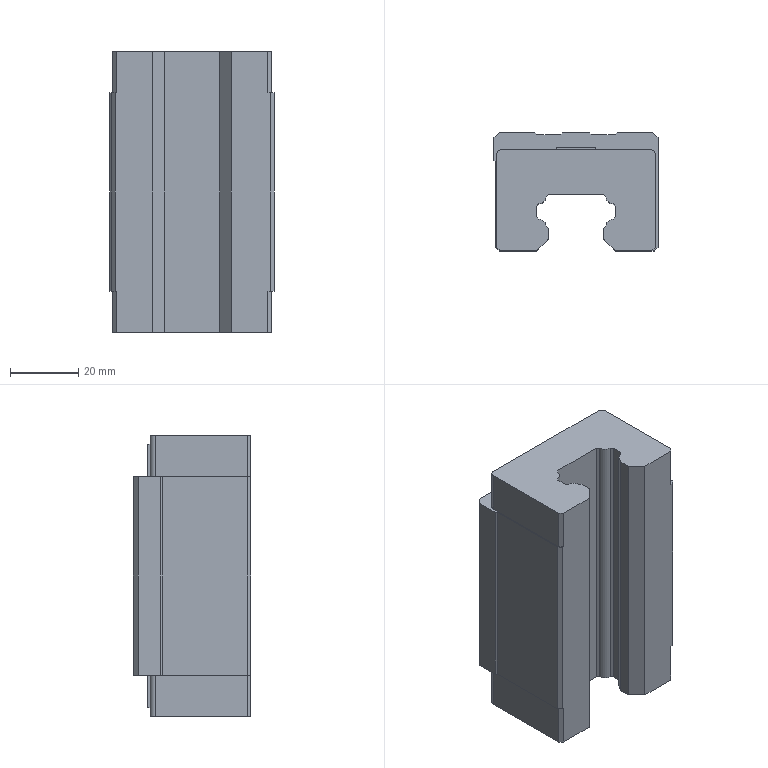Part | STEP file | HGH25 Slider | 1 solid | 80 faces | box 48 x 34.5 x 82 mm | volume 100220 mm3 | plane 56 | cylinder 16 | cone 8 | commonest cylinder face diameters 6 x8 3 x4 4.6 x4